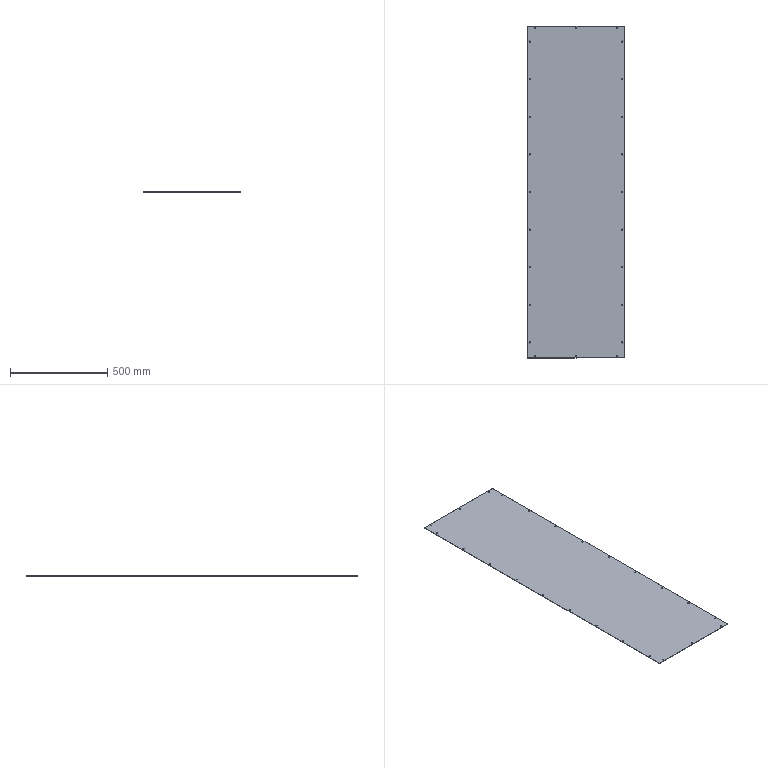Part | SolidWorks | 1 solid | 54 faces | box 494.5 x 1703 x 2 mm | volume 1682674 mm3 | cylinder 48 | plane 6 | commonest cylinder face diameters 6.5 x48